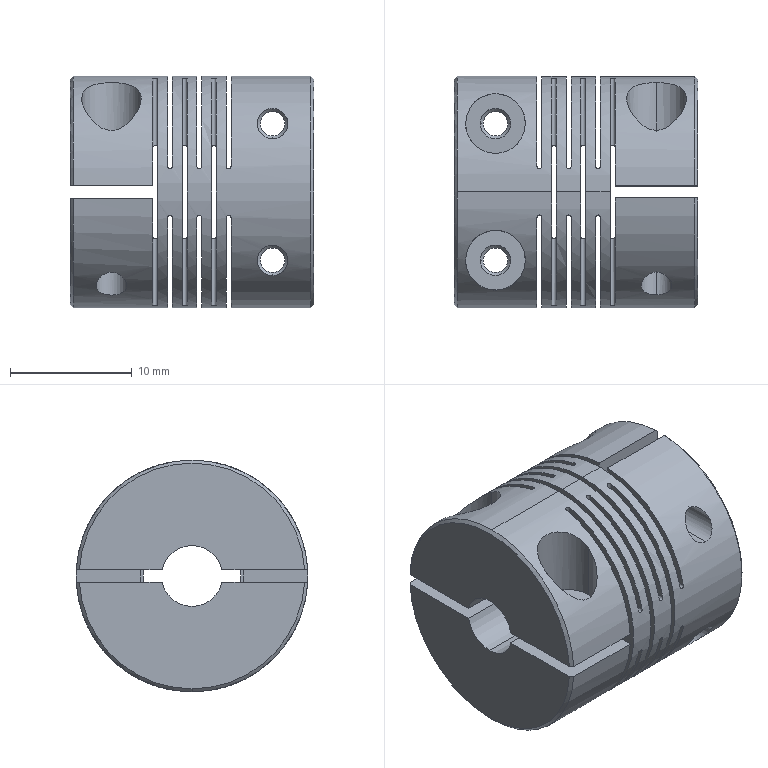Part | SolidWorks | features BaseBody 1 | 1 solid | 132 faces | box 20 x 19 x 19 mm | volume 3713 mm3 | cylinder 71 | plane 40 | cone 21 | commonest cylinder face diameters 0.4 x30 2.5 x16 2.013 x8 4.9 x8 5 x3 8 x2